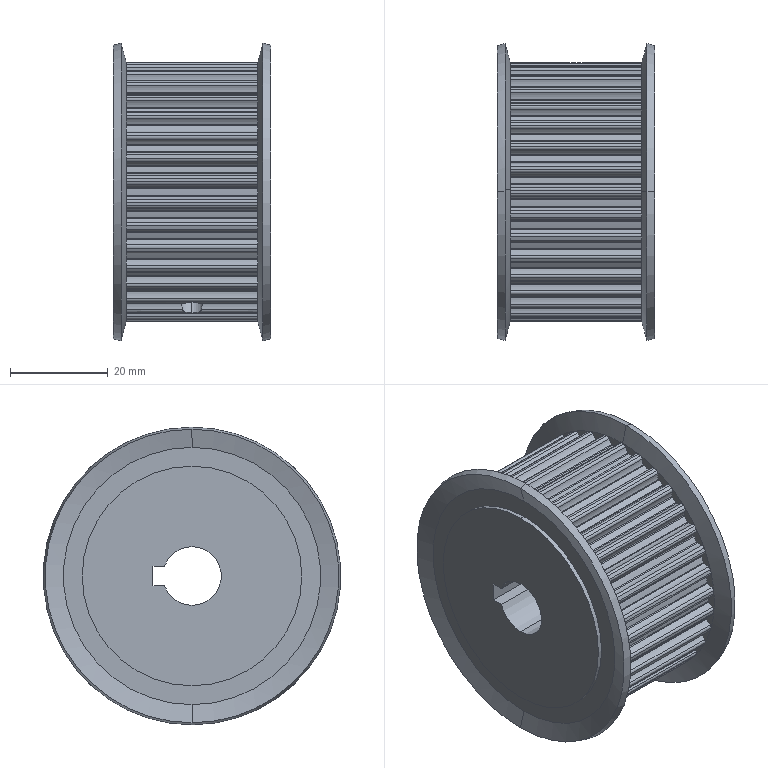Part | STEP file | HTPA34S5M250-A-N12 high-torque timing pulley MISUMI 110 | 1 solid | 386 faces | box 32.194 x 61 x 61 mm | volume 63360 mm3 | cylinder 298 | plane 76 | cone 12 | commonest cylinder face diameters 0.5 x72 1.1 x72 6.55 x72 49.61 x36 53.15 x34 4.917 x4